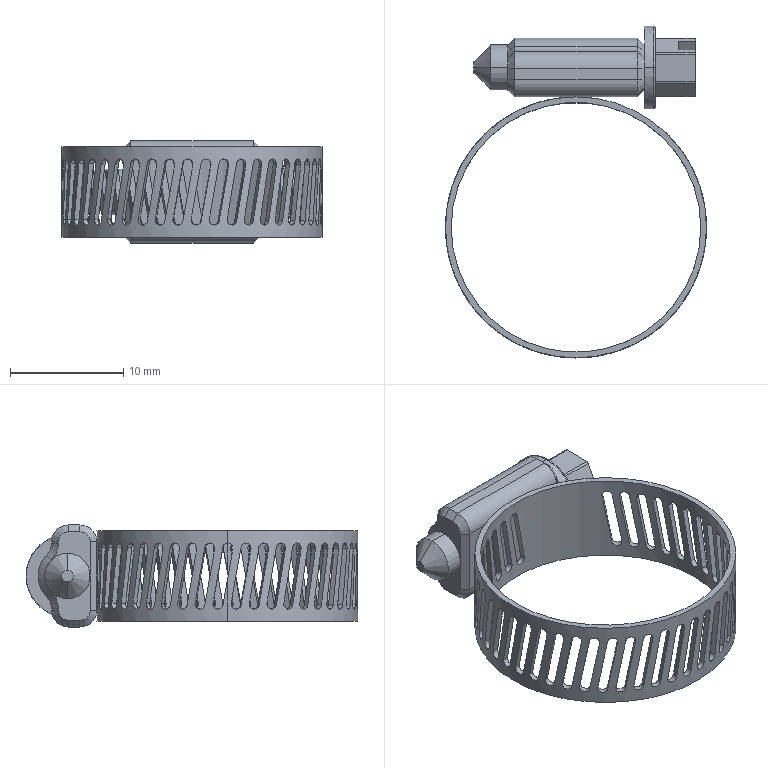Part | SolidWorks | features ICE 7, Chamfer 2, Fillet 2, CirPattern 1, ExtruThin 1 | 2 solids | 306 faces | box 23 x 29.251 x 9 mm | volume 732.821 mm3 | cylinder 157 | plane 131 | cone 16 | torus 2 | commonest cylinder face diameters 0.9 x120 0.4 x22 3 x6 4 x2 7.3 x2 22 x2